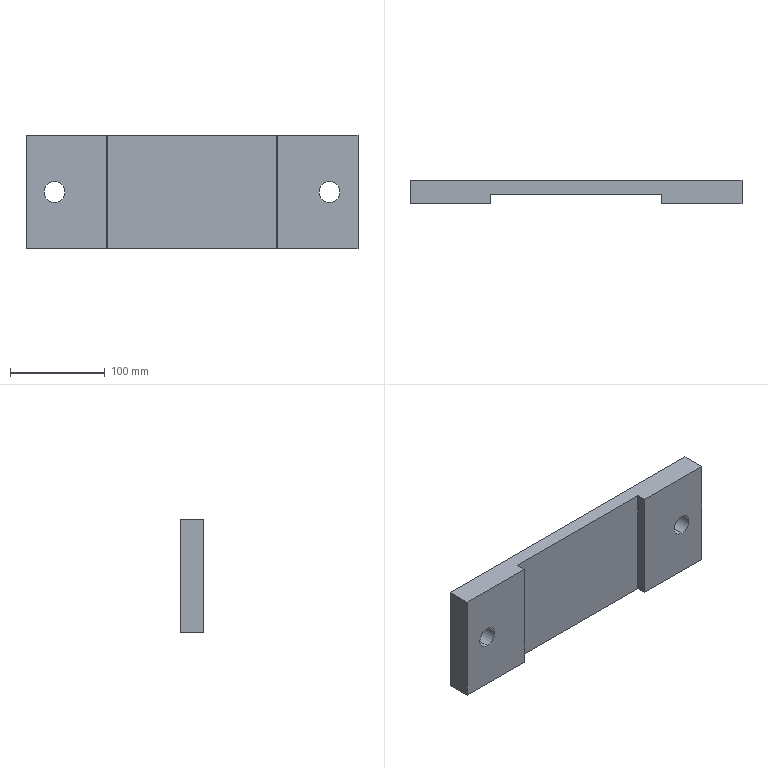Part | SolidWorks | features ICE 2, Extrusion 1, Fillet 1 | 1 solid | 16 faces | box 350 x 25 x 120 mm | volume 815006 mm3 | plane 10 | cylinder 6 | commonest cylinder face diameters 22 x4 1 x2
STEP:
#1=CARTESIAN_POINT('',(145.,0.,-11.));
#2=VERTEX_POINT('',#1);
#3=CARTESIAN_POINT('',(145.,0.,11.));
#4=VERTEX_POINT('',#3);
#5=CARTESIAN_POINT('',(145.,0.,0.));
#6=DIRECTION('',(0.,1.,0.));
#7=DIRECTION('',(0.,0.,-1.));
#8=AXIS2_PLACEMENT_3D('',#5,#6,#7);
#9=CIRCLE('',#8,11.);
#10=EDGE_CURVE('',#2,#4,#9,.T.);
#11=ORIENTED_EDGE('',*,*,#10,.F.);
#12=CARTESIAN_POINT('',(145.,25.,-11.));
#13=VERTEX_POINT('',#12);
#14=CARTESIAN_POINT('',(145.,0.,-11.));
#15=DIRECTION('',(0.,1.,0.));
#16=VECTOR('',#15,1000.);
#17=LINE('',#14,#16);
#18=EDGE_CURVE('',#2,#13,#17,.T.);
#19=ORIENTED_EDGE('',*,*,#18,.T.);
#20=CARTESIAN_POINT('',(145.,25.,11.));
#21=VERTEX_POINT('',#20);
#22=CARTESIAN_POINT('',(145.,25.,0.));
#23=DIRECTION('',(0.,1.,0.));
#24=DIRECTION('',(0.,0.,-1.));
#25=AXIS2_PLACEMENT_3D('',#22,#23,#24);
#26=CIRCLE('',#25,11.);
#27=EDGE_CURVE('',#13,#21,#26,.T.);
#28=ORIENTED_EDGE('',*,*,#27,.T.);
#29=CARTESIAN_POINT('',(145.,0.,11.));
#30=DIRECTION('',(0.,1.,0.));
#31=VECTOR('',#30,1000.);
#32=LINE('',#29,#31);
#33=EDGE_CURVE('',#4,#21,#32,.T.);
#34=ORIENTED_EDGE('',*,*,#33,.F.);
#35=EDGE_LOOP('',(#11,#19,#28,#34));
#36=FACE_OUTER_BOUND('',#35,.T.);
#37=CARTESIAN_POINT('',(145.,0.,0.));
#38=DIRECTION('',(0.,1.,0.));
#39=DIRECTION('',(0.,0.,1.));
#40=AXIS2_PLACEMENT_3D('',#37,#38,#39);
#41=CYLINDRICAL_SURFACE('',#40,11.);
#42=ADVANCED_FACE('',(#36),#41,.F.);
#43=CARTESIAN_POINT('',(-145.,0.,-11.));
#44=VERTEX_POINT('',#43);
#45=CARTESIAN_POINT('',(-145.,0.,11.));
#46=VERTEX_POINT('',#45);
#47=CARTESIAN_POINT('',(-145.,0.,0.));
#48=DIRECTION('',(0.,1.,0.));
#49=DIRECTION('',(0.,0.,1.));
#50=AXIS2_PLACEMENT_3D('',#47,#48,#49);
#51=CIRCLE('',#50,11.);
#52=EDGE_CURVE('',#44,#46,#51,.T.);
#53=ORIENTED_EDGE('',*,*,#52,.F.);
#54=CARTESIAN_POINT('',(-145.,25.,-11.));
#55=VERTEX_POINT('',#54);
#56=CARTESIAN_POINT('',(-145.,0.,-11.));
#57=DIRECTION('',(0.,1.,0.));
#58=VECTOR('',#57,1000.);
#59=LINE('',#56,#58);
#60=EDGE_CURVE('',#44,#55,#59,.T.);
#61=ORIENTED_EDGE('',*,*,#60,.T.);
#62=CARTESIAN_POINT('',(-145.,25.,11.));
#63=VERTEX_POINT('',#62);
#64=CARTESIAN_POINT('',(-145.,25.,0.));
#65=DIRECTION('',(0.,1.,0.));
#66=DIRECTION('',(0.,0.,1.));
#67=AXIS2_PLACEMENT_3D('',#64,#65,#66);
#68=CIRCLE('',#67,11.);
#69=EDGE_CURVE('',#55,#63,#68,.T.);
#70=ORIENTED_EDGE('',*,*,#69,.T.);
#71=CARTESIAN_POINT('',(-145.,0.,11.));
#72=DIRECTION('',(0.,1.,0.));
#73=VECTOR('',#72,1000.);
#74=LINE('',#71,#73);
#75=EDGE_CURVE('',#46,#63,#74,.T.);
#76=ORIENTED_EDGE('',*,*,#75,.F.);
#77=EDGE_LOOP('',(#53,#61,#70,#76));
#78=FACE_OUTER_BOUND('',#77,.T.);
#79=CARTESIAN_POINT('',(-145.,0.,0.));
#80=DIRECTION('',(0.,1.,0.));
#81=DIRECTION('',(0.,0.,1.));
#82=AXIS2_PLACEMENT_3D('',#79,#80,#81);
#83=CYLINDRICAL_SURFACE('',#82,11.);
#84=ADVANCED_FACE('',(#78),#83,.F.);
#85=CARTESIAN_POINT('',(145.,0.,0.));
#86=DIRECTION('',(0.,1.,0.));
#87=DIRECTION('',(0.,0.,-1.));
#88=AXIS2_PLACEMENT_3D('',#85,#86,#87);
#89=CIRCLE('',#88,11.);
#90=EDGE_CURVE('',#4,#2,#89,.T.);
#91=ORIENTED_EDGE('',*,*,#90,.T.);
#92=ORIENTED_EDGE('',*,*,#10,.T.);
#93=EDGE_LOOP('',(#91,#92));
#94=FACE_BOUND('',#93,.T.);
#95=CARTESIAN_POINT('',(90.,0.,60.));
#96=VERTEX_POINT('',#95);
#97=CARTESIAN_POINT('',(175.,0.,60.));
#98=VERTEX_POINT('',#97);
#99=CARTESIAN_POINT('',(-175.,0.,60.));
#100=DIRECTION('',(1.,0.,0.));
#101=VECTOR('',#100,1000.);
#102=LINE('',#99,#101);
#103=EDGE_CURVE('',#96,#98,#102,.T.);
#104=ORIENTED_EDGE('',*,*,#103,.F.);
#105=CARTESIAN_POINT('',(90.,0.,-60.));
#106=VERTEX_POINT('',#105);
#107=CARTESIAN_POINT('',(90.,0.,0.));
#108=DIRECTION('',(0.,0.,-1.));
#109=VECTOR('',#108,1000.);
#110=LINE('',#107,#109);
#111=EDGE_CURVE('',#96,#106,#110,.T.);
#112=ORIENTED_EDGE('',*,*,#111,.T.);
#113=CARTESIAN_POINT('',(175.,0.,-60.));
#114=VERTEX_POINT('',#113);
#115=CARTESIAN_POINT('',(-175.,0.,-60.));
#116=DIRECTION('',(-1.,0.,0.));
#117=VECTOR('',#116,1000.);
#118=LINE('',#115,#117);
#119=EDGE_CURVE('',#114,#106,#118,.T.);
#120=ORIENTED_EDGE('',*,*,#119,.F.);
#121=CARTESIAN_POINT('',(175.,0.,-60.));
#122=DIRECTION('',(0.,0.,-1.));
#123=VECTOR('',#122,1000.);
#124=LINE('',#121,#123);
#125=EDGE_CURVE('',#98,#114,#124,.T.);
#126=ORIENTED_EDGE('',*,*,#125,.F.);
#127=EDGE_LOOP('',(#104,#112,#120,#126));
#128=FACE_OUTER_BOUND('',#127,.T.);
#129=CARTESIAN_POINT('',(0.,0.,0.));
#130=DIRECTION('',(0.,1.,0.));
#131=DIRECTION('',(0.,0.,1.));
#132=AXIS2_PLACEMENT_3D('',#129,#130,#131);
#133=PLANE('',#132);
#134=ADVANCED_FACE('',(#94,#128),#133,.F.);
#135=ORIENTED_EDGE('',*,*,#125,.T.);
#136=CARTESIAN_POINT('',(175.,25.,-60.));
#137=VERTEX_POINT('',#136);
#138=CARTESIAN_POINT('',(175.,25.,-60.));
#139=DIRECTION('',(0.,-1.,0.));
#140=VECTOR('',#139,1000.);
#141=LINE('',#138,#140);
#142=EDGE_CURVE('',#137,#114,#141,.T.);
#143=ORIENTED_EDGE('',*,*,#142,.F.);
#144=CARTESIAN_POINT('',(175.,25.,60.));
#145=VERTEX_POINT('',#144);
#146=CARTESIAN_POINT('',(175.,25.,-60.));
#147=DIRECTION('',(0.,0.,-1.));
#148=VECTOR('',#147,1000.);
#149=LINE('',#146,#148);
#150=EDGE_CURVE('',#145,#137,#149,.T.);
#151=ORIENTED_EDGE('',*,*,#150,.F.);
#152=CARTESIAN_POINT('',(175.,25.,60.));
#153=DIRECTION('',(0.,-1.,0.));
#154=VECTOR('',#153,1000.);
#155=LINE('',#152,#154);
#156=EDGE_CURVE('',#145,#98,#155,.T.);
#157=ORIENTED_EDGE('',*,*,#156,.T.);
#158=EDGE_LOOP('',(#135,#143,#151,#157));
#159=FACE_OUTER_BOUND('',#158,.T.);
#160=CARTESIAN_POINT('',(175.,25.,-60.));
#161=DIRECTION('',(-1.,0.,0.));
#162=DIRECTION('',(0.,0.,1.));
#163=AXIS2_PLACEMENT_3D('',#160,#161,#162);
#164=PLANE('',#163);
#165=ADVANCED_FACE('',(#159),#164,.F.);
#166=ORIENTED_EDGE('',*,*,#119,.T.);
#167=CARTESIAN_POINT('',(90.,9.5,-60.));
#168=VERTEX_POINT('',#167);
#169=CARTESIAN_POINT('',(90.,-10.,-60.));
#170=DIRECTION('',(0.,1.,0.));
#171=VECTOR('',#170,1000.);
#172=LINE('',#169,#171);
#173=EDGE_CURVE('',#106,#168,#172,.T.);
#174=ORIENTED_EDGE('',*,*,#173,.T.);
#175=CARTESIAN_POINT('',(89.5,10.,-60.));
#176=VERTEX_POINT('',#175);
#177=CARTESIAN_POINT('',(89.5,9.5,-60.));
#178=DIRECTION('',(0.,0.,1.));
#179=DIRECTION('',(1.,0.,0.));
#180=AXIS2_PLACEMENT_3D('',#177,#178,#179);
#181=CIRCLE('',#180,0.5);
#182=EDGE_CURVE('',#168,#176,#181,.T.);
#183=ORIENTED_EDGE('',*,*,#182,.T.);
#184=CARTESIAN_POINT('',(-89.5,10.,-60.));
#185=VERTEX_POINT('',#184);
#186=CARTESIAN_POINT('',(-90.,10.,-60.));
#187=DIRECTION('',(-1.,0.,0.));
#188=VECTOR('',#187,1000.);
#189=LINE('',#186,#188);
#190=EDGE_CURVE('',#176,#185,#189,.T.);
#191=ORIENTED_EDGE('',*,*,#190,.T.);
#192=CARTESIAN_POINT('',(-90.,9.5,-60.));
#193=VERTEX_POINT('',#192);
#194=CARTESIAN_POINT('',(-89.5,9.5,-60.));
#195=DIRECTION('',(0.,0.,1.));
#196=DIRECTION('',(1.,0.,0.));
#197=AXIS2_PLACEMENT_3D('',#194,#195,#196);
#198=CIRCLE('',#197,0.5);
#199=EDGE_CURVE('',#185,#193,#198,.T.);
#200=ORIENTED_EDGE('',*,*,#199,.T.);
#201=CARTESIAN_POINT('',(-90.,0.,-60.));
#202=VERTEX_POINT('',#201);
#203=CARTESIAN_POINT('',(-90.,-10.,-60.));
#204=DIRECTION('',(0.,-1.,0.));
#205=VECTOR('',#204,1000.);
#206=LINE('',#203,#205);
#207=EDGE_CURVE('',#193,#202,#206,.T.);
#208=ORIENTED_EDGE('',*,*,#207,.T.);
#209=CARTESIAN_POINT('',(-175.,0.,-60.));
#210=VERTEX_POINT('',#209);
#211=CARTESIAN_POINT('',(-175.,0.,-60.));
#212=DIRECTION('',(-1.,0.,0.));
#213=VECTOR('',#212,1000.);
#214=LINE('',#211,#213);
#215=EDGE_CURVE('',#202,#210,#214,.T.);
#216=ORIENTED_EDGE('',*,*,#215,.T.);
#217=CARTESIAN_POINT('',(-175.,25.,-60.));
#218=VERTEX_POINT('',#217);
#219=CARTESIAN_POINT('',(-175.,25.,-60.));
#220=DIRECTION('',(0.,-1.,0.));
#221=VECTOR('',#220,1000.);
#222=LINE('',#219,#221);
#223=EDGE_CURVE('',#218,#210,#222,.T.);
#224=ORIENTED_EDGE('',*,*,#223,.F.);
#225=CARTESIAN_POINT('',(-175.,25.,-60.));
#226=DIRECTION('',(-1.,0.,0.));
#227=VECTOR('',#226,1000.);
#228=LINE('',#225,#227);
#229=EDGE_CURVE('',#137,#218,#228,.T.);
#230=ORIENTED_EDGE('',*,*,#229,.F.);
#231=ORIENTED_EDGE('',*,*,#142,.T.);
#232=EDGE_LOOP('',(#166,#174,#183,#191,#200,#208,#216,#224,#230,#231));
#233=FACE_OUTER_BOUND('',#232,.T.);
#234=CARTESIAN_POINT('',(-175.,25.,-60.));
#235=DIRECTION('',(0.,0.,1.));
#236=DIRECTION('',(1.,0.,0.));
#237=AXIS2_PLACEMENT_3D('',#234,#235,#236);
#238=PLANE('',#237);
#239=ADVANCED_FACE('',(#233),#238,.F.);
#240=CARTESIAN_POINT('',(-175.,0.,60.));
#241=VERTEX_POINT('',#240);
#242=CARTESIAN_POINT('',(-175.,0.,-60.));
#243=DIRECTION('',(0.,0.,1.));
#244=VECTOR('',#243,1000.);
#245=LINE('',#242,#244);
#246=EDGE_CURVE('',#210,#241,#245,.T.);
#247=ORIENTED_EDGE('',*,*,#246,.T.);
#248=CARTESIAN_POINT('',(-175.,25.,60.));
#249=VERTEX_POINT('',#248);
#250=CARTESIAN_POINT('',(-175.,25.,60.));
#251=DIRECTION('',(0.,-1.,0.));
#252=VECTOR('',#251,1000.);
#253=LINE('',#250,#252);
#254=EDGE_CURVE('',#249,#241,#253,.T.);
#255=ORIENTED_EDGE('',*,*,#254,.F.);
#256=CARTESIAN_POINT('',(-175.,25.,-60.));
#257=DIRECTION('',(0.,0.,1.));
#258=VECTOR('',#257,1000.);
#259=LINE('',#256,#258);
#260=EDGE_CURVE('',#218,#249,#259,.T.);
#261=ORIENTED_EDGE('',*,*,#260,.F.);
#262=ORIENTED_EDGE('',*,*,#223,.T.);
#263=EDGE_LOOP('',(#247,#255,#261,#262));
#264=FACE_OUTER_BOUND('',#263,.T.);
#265=CARTESIAN_POINT('',(-175.,25.,-60.));
#266=DIRECTION('',(1.,0.,0.));
#267=DIRECTION('',(0.,0.,-1.));
#268=AXIS2_PLACEMENT_3D('',#265,#266,#267);
#269=PLANE('',#268);
#270=ADVANCED_FACE('',(#264),#269,.F.);
#271=CARTESIAN_POINT('',(89.5,10.,60.));
#272=VERTEX_POINT('',#271);
#273=CARTESIAN_POINT('',(-89.5,10.,60.));
#274=VERTEX_POINT('',#273);
#275=CARTESIAN_POINT('',(-90.,10.,60.));
#276=DIRECTION('',(-1.,0.,0.));
#277=VECTOR('',#276,1000.);
#278=LINE('',#275,#277);
#279=EDGE_CURVE('',#272,#274,#278,.T.);
#280=ORIENTED_EDGE('',*,*,#279,.F.);
#281=CARTESIAN_POINT('',(90.,9.5,60.));
#282=VERTEX_POINT('',#281);
#283=CARTESIAN_POINT('',(89.5,9.5,60.));
#284=DIRECTION('',(0.,0.,-1.));
#285=DIRECTION('',(-1.,0.,0.));
#286=AXIS2_PLACEMENT_3D('',#283,#284,#285);
#287=CIRCLE('',#286,0.5);
#288=EDGE_CURVE('',#272,#282,#287,.T.);
#289=ORIENTED_EDGE('',*,*,#288,.T.);
#290=CARTESIAN_POINT('',(90.,-10.,60.));
#291=DIRECTION('',(0.,1.,0.));
#292=VECTOR('',#291,1000.);
#293=LINE('',#290,#292);
#294=EDGE_CURVE('',#96,#282,#293,.T.);
#295=ORIENTED_EDGE('',*,*,#294,.F.);
#296=ORIENTED_EDGE('',*,*,#103,.T.);
#297=ORIENTED_EDGE('',*,*,#156,.F.);
#298=CARTESIAN_POINT('',(-175.,25.,60.));
#299=DIRECTION('',(1.,0.,0.));
#300=VECTOR('',#299,1000.);
#301=LINE('',#298,#300);
#302=EDGE_CURVE('',#249,#145,#301,.T.);
#303=ORIENTED_EDGE('',*,*,#302,.F.);
#304=ORIENTED_EDGE('',*,*,#254,.T.);
#305=CARTESIAN_POINT('',(-90.,0.,60.));
#306=VERTEX_POINT('',#305);
#307=CARTESIAN_POINT('',(-175.,0.,60.));
#308=DIRECTION('',(1.,0.,0.));
#309=VECTOR('',#308,1000.);
#310=LINE('',#307,#309);
#311=EDGE_CURVE('',#241,#306,#310,.T.);
#312=ORIENTED_EDGE('',*,*,#311,.T.);
#313=CARTESIAN_POINT('',(-90.,9.5,60.));
#314=VERTEX_POINT('',#313);
#315=CARTESIAN_POINT('',(-90.,-10.,60.));
#316=DIRECTION('',(0.,-1.,0.));
#317=VECTOR('',#316,1000.);
#318=LINE('',#315,#317);
#319=EDGE_CURVE('',#314,#306,#318,.T.);
#320=ORIENTED_EDGE('',*,*,#319,.F.);
#321=CARTESIAN_POINT('',(-89.5,9.5,60.));
#322=DIRECTION('',(0.,0.,-1.));
#323=DIRECTION('',(-1.,0.,0.));
#324=AXIS2_PLACEMENT_3D('',#321,#322,#323);
#325=CIRCLE('',#324,0.5);
#326=EDGE_CURVE('',#314,#274,#325,.T.);
#327=ORIENTED_EDGE('',*,*,#326,.T.);
#328=EDGE_LOOP('',(#280,#289,#295,#296,#297,#303,#304,#312,#320,#327));
#329=FACE_OUTER_BOUND('',#328,.T.);
#330=CARTESIAN_POINT('',(-175.,25.,60.));
#331=DIRECTION('',(0.,0.,-1.));
#332=DIRECTION('',(-1.,0.,0.));
#333=AXIS2_PLACEMENT_3D('',#330,#331,#332);
#334=PLANE('',#333);
#335=ADVANCED_FACE('',(#329),#334,.F.);
#336=CARTESIAN_POINT('',(-145.,25.,0.));
#337=DIRECTION('',(0.,1.,0.));
#338=DIRECTION('',(0.,0.,1.));
#339=AXIS2_PLACEMENT_3D('',#336,#337,#338);
#340=CIRCLE('',#339,11.);
#341=EDGE_CURVE('',#63,#55,#340,.T.);
#342=ORIENTED_EDGE('',*,*,#341,.F.);
#343=ORIENTED_EDGE('',*,*,#69,.F.);
#344=EDGE_LOOP('',(#342,#343));
#345=FACE_BOUND('',#344,.T.);
#346=CARTESIAN_POINT('',(145.,25.,0.));
#347=DIRECTION('',(0.,1.,0.));
#348=DIRECTION('',(0.,0.,-1.));
#349=AXIS2_PLACEMENT_3D('',#346,#347,#348);
#350=CIRCLE('',#349,11.);
#351=EDGE_CURVE('',#21,#13,#350,.T.);
#352=ORIENTED_EDGE('',*,*,#351,.F.);
#353=ORIENTED_EDGE('',*,*,#27,.F.);
#354=EDGE_LOOP('',(#352,#353));
#355=FACE_BOUND('',#354,.T.);
#356=ORIENTED_EDGE('',*,*,#150,.T.);
#357=ORIENTED_EDGE('',*,*,#229,.T.);
#358=ORIENTED_EDGE('',*,*,#260,.T.);
#359=ORIENTED_EDGE('',*,*,#302,.T.);
#360=EDGE_LOOP('',(#356,#357,#358,#359));
#361=FACE_OUTER_BOUND('',#360,.T.);
#362=CARTESIAN_POINT('',(0.,25.,0.));
#363=DIRECTION('',(0.,1.,0.));
#364=DIRECTION('',(0.,0.,1.));
#365=AXIS2_PLACEMENT_3D('',#362,#363,#364);
#366=PLANE('',#365);
#367=ADVANCED_FACE('',(#345,#355,#361),#366,.T.);
#368=CARTESIAN_POINT('',(-145.,0.,0.));
#369=DIRECTION('',(0.,1.,0.));
#370=DIRECTION('',(0.,0.,1.));
#371=AXIS2_PLACEMENT_3D('',#368,#369,#370);
#372=CIRCLE('',#371,11.);
#373=EDGE_CURVE('',#46,#44,#372,.T.);
#374=ORIENTED_EDGE('',*,*,#373,.T.);
#375=ORIENTED_EDGE('',*,*,#52,.T.);
#376=EDGE_LOOP('',(#374,#375));
#377=FACE_BOUND('',#376,.T.);
#378=ORIENTED_EDGE('',*,*,#215,.F.);
#379=CARTESIAN_POINT('',(-90.,0.,0.));
#380=DIRECTION('',(0.,0.,1.));
#381=VECTOR('',#380,1000.);
#382=LINE('',#379,#381);
#383=EDGE_CURVE('',#202,#306,#382,.T.);
#384=ORIENTED_EDGE('',*,*,#383,.T.);
#385=ORIENTED_EDGE('',*,*,#311,.F.);
#386=ORIENTED_EDGE('',*,*,#246,.F.);
#387=EDGE_LOOP('',(#378,#384,#385,#386));
#388=FACE_OUTER_BOUND('',#387,.T.);
#389=CARTESIAN_POINT('',(0.,0.,0.));
#390=DIRECTION('',(0.,1.,0.));
#391=DIRECTION('',(0.,0.,1.));
#392=AXIS2_PLACEMENT_3D('',#389,#390,#391);
#393=PLANE('',#392);
#394=ADVANCED_FACE('',(#377,#388),#393,.F.);
#395=ORIENTED_EDGE('',*,*,#294,.T.);
#396=CARTESIAN_POINT('',(90.,9.5,-60.));
#397=DIRECTION('',(0.,0.,-1.));
#398=VECTOR('',#397,1000.);
#399=LINE('',#396,#398);
#400=EDGE_CURVE('',#282,#168,#399,.T.);
#401=ORIENTED_EDGE('',*,*,#400,.T.);
#402=ORIENTED_EDGE('',*,*,#173,.F.);
#403=ORIENTED_EDGE('',*,*,#111,.F.);
#404=EDGE_LOOP('',(#395,#401,#402,#403));
#405=FACE_OUTER_BOUND('',#404,.T.);
#406=CARTESIAN_POINT('',(90.,-10.,-60.));
#407=DIRECTION('',(1.,0.,0.));
#408=DIRECTION('',(0.,0.,-1.));
#409=AXIS2_PLACEMENT_3D('',#406,#407,#408);
#410=PLANE('',#409);
#411=ADVANCED_FACE('',(#405),#410,.F.);
#412=ORIENTED_EDGE('',*,*,#207,.F.);
#413=CARTESIAN_POINT('',(-90.,9.5,60.));
#414=DIRECTION('',(0.,0.,1.));
#415=VECTOR('',#414,1000.);
#416=LINE('',#413,#415);
#417=EDGE_CURVE('',#193,#314,#416,.T.);
#418=ORIENTED_EDGE('',*,*,#417,.T.);
#419=ORIENTED_EDGE('',*,*,#319,.T.);
#420=ORIENTED_EDGE('',*,*,#383,.F.);
#421=EDGE_LOOP('',(#412,#418,#419,#420));
#422=FACE_OUTER_BOUND('',#421,.T.);
#423=CARTESIAN_POINT('',(-90.,-10.,-60.));
#424=DIRECTION('',(-1.,0.,0.));
#425=DIRECTION('',(0.,0.,1.));
#426=AXIS2_PLACEMENT_3D('',#423,#424,#425);
#427=PLANE('',#426);
#428=ADVANCED_FACE('',(#422),#427,.F.);
#429=ORIENTED_EDGE('',*,*,#190,.F.);
#430=CARTESIAN_POINT('',(89.5,10.,60.));
#431=DIRECTION('',(0.,0.,1.));
#432=VECTOR('',#431,1000.);
#433=LINE('',#430,#432);
#434=EDGE_CURVE('',#176,#272,#433,.T.);
#435=ORIENTED_EDGE('',*,*,#434,.T.);
#436=ORIENTED_EDGE('',*,*,#279,.T.);
#437=CARTESIAN_POINT('',(-89.5,10.,-60.));
#438=DIRECTION('',(0.,0.,-1.));
#439=VECTOR('',#438,1000.);
#440=LINE('',#437,#439);
#441=EDGE_CURVE('',#274,#185,#440,.T.);
#442=ORIENTED_EDGE('',*,*,#441,.T.);
#443=EDGE_LOOP('',(#429,#435,#436,#442));
#444=FACE_OUTER_BOUND('',#443,.T.);
#445=CARTESIAN_POINT('',(-90.,10.,-60.));
#446=DIRECTION('',(0.,1.,0.));
#447=DIRECTION('',(0.,0.,1.));
#448=AXIS2_PLACEMENT_3D('',#445,#446,#447);
#449=PLANE('',#448);
#450=ADVANCED_FACE('',(#444),#449,.F.);
#451=ORIENTED_EDGE('',*,*,#60,.F.);
#452=ORIENTED_EDGE('',*,*,#373,.F.);
#453=ORIENTED_EDGE('',*,*,#75,.T.);
#454=ORIENTED_EDGE('',*,*,#341,.T.);
#455=EDGE_LOOP('',(#451,#452,#453,#454));
#456=FACE_OUTER_BOUND('',#455,.T.);
#457=CARTESIAN_POINT('',(-145.,0.,0.));
#458=DIRECTION('',(0.,1.,0.));
#459=DIRECTION('',(0.,0.,1.));
#460=AXIS2_PLACEMENT_3D('',#457,#458,#459);
#461=CYLINDRICAL_SURFACE('',#460,11.);
#462=ADVANCED_FACE('',(#456),#461,.F.);
#463=ORIENTED_EDGE('',*,*,#18,.F.);
#464=ORIENTED_EDGE('',*,*,#90,.F.);
#465=ORIENTED_EDGE('',*,*,#33,.T.);
#466=ORIENTED_EDGE('',*,*,#351,.T.);
#467=EDGE_LOOP('',(#463,#464,#465,#466));
#468=FACE_OUTER_BOUND('',#467,.T.);
#469=CARTESIAN_POINT('',(145.,0.,0.));
#470=DIRECTION('',(0.,1.,0.));
#471=DIRECTION('',(0.,0.,1.));
#472=AXIS2_PLACEMENT_3D('',#469,#470,#471);
#473=CYLINDRICAL_SURFACE('',#472,11.);
#474=ADVANCED_FACE('',(#468),#473,.F.);
#475=ORIENTED_EDGE('',*,*,#182,.F.);
#476=ORIENTED_EDGE('',*,*,#400,.F.);
#477=ORIENTED_EDGE('',*,*,#288,.F.);
#478=ORIENTED_EDGE('',*,*,#434,.F.);
#479=EDGE_LOOP('',(#475,#476,#477,#478));
#480=FACE_OUTER_BOUND('',#479,.T.);
#481=CARTESIAN_POINT('',(89.5,9.5,-60.));
#482=DIRECTION('',(0.,0.,-1.));
#483=DIRECTION('',(-1.,0.,0.));
#484=AXIS2_PLACEMENT_3D('',#481,#482,#483);
#485=CYLINDRICAL_SURFACE('',#484,0.5);
#486=ADVANCED_FACE('',(#480),#485,.F.);
#487=ORIENTED_EDGE('',*,*,#199,.F.);
#488=ORIENTED_EDGE('',*,*,#441,.F.);
#489=ORIENTED_EDGE('',*,*,#326,.F.);
#490=ORIENTED_EDGE('',*,*,#417,.F.);
#491=EDGE_LOOP('',(#487,#488,#489,#490));
#492=FACE_OUTER_BOUND('',#491,.T.);
#493=CARTESIAN_POINT('',(-89.5,9.5,-60.));
#494=DIRECTION('',(0.,0.,-1.));
#495=DIRECTION('',(-1.,0.,0.));
#496=AXIS2_PLACEMENT_3D('',#493,#494,#495);
#497=CYLINDRICAL_SURFACE('',#496,0.5);
#498=ADVANCED_FACE('',(#492),#497,.F.);
#499=CLOSED_SHELL('',(#42,#84,#134,#165,#239,#270,#335,#367,#394,#411,#428,#450,#462,#474,#486,#498));
#500=MANIFOLD_SOLID_BREP('',#499);
#501=CARTESIAN_POINT('',(0.,0.,0.));
#502=DIRECTION('',(0.,0.,1.));
#503=DIRECTION('',(1.,0.,0.));
#504=AXIS2_PLACEMENT_3D('',#501,#502,#503);
#505=(LENGTH_UNIT()NAMED_UNIT(*)SI_UNIT(.MILLI.,.METRE.));
#506=UNCERTAINTY_MEASURE_WITH_UNIT(LENGTH_MEASURE(0.00001),#505,'','');
#507=(NAMED_UNIT(*)PLANE_ANGLE_UNIT()SI_UNIT($,.RADIAN.));
#508=(NAMED_UNIT(*)SI_UNIT($,.STERADIAN.)SOLID_ANGLE_UNIT());
#509=(GEOMETRIC_REPRESENTATION_CONTEXT(3)GLOBAL_UNCERTAINTY_ASSIGNED_CONTEXT((#506))GLOBAL_UNIT_ASSIGNED_CONTEXT((#505,#507,#508))REPRESENTATION_CONTEXT('',''));
#510=ADVANCED_BREP_SHAPE_REPRESENTATION('',(#500,#504),#509);